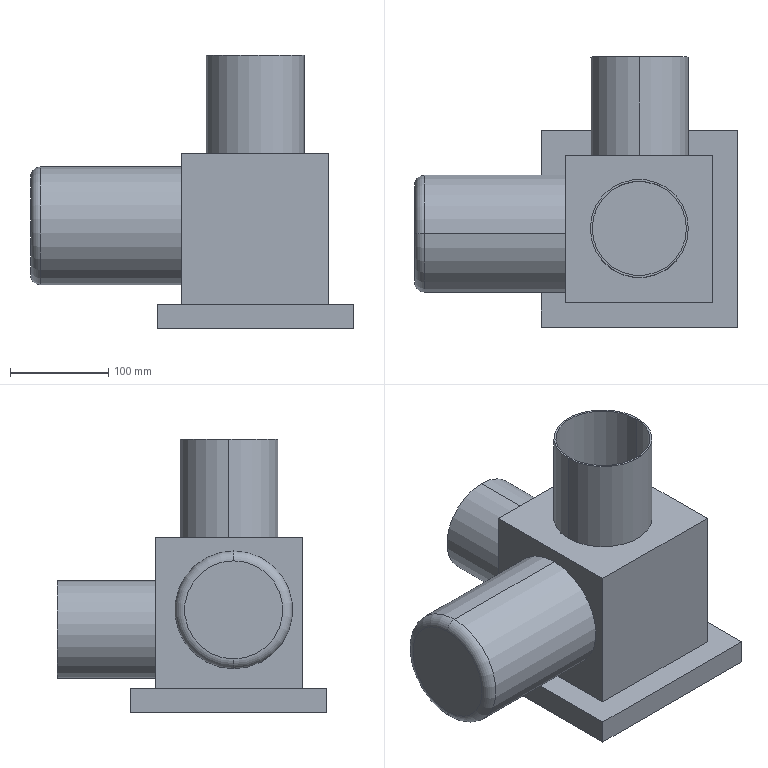Part | SolidWorks | features ICE 5, Extrusion 1, Fillet 1 | 1 solid | 28 faces | box 329 x 275 x 279 mm | volume 6409711 mm3 | plane 16 | cylinder 10 | torus 2 | commonest cylinder face diameters 100 x4 90 x2 96 x2 120 x2
STEP:
#1=CARTESIAN_POINT('',(-48.,0.,179.));
#2=VERTEX_POINT('',#1);
#3=CARTESIAN_POINT('',(48.,0.,179.));
#4=VERTEX_POINT('',#3);
#5=CARTESIAN_POINT('',(0.,0.,179.));
#6=DIRECTION('',(0.,0.,1.));
#7=DIRECTION('',(-1.,0.,0.));
#8=AXIS2_PLACEMENT_3D('',#5,#6,#7);
#9=CIRCLE('',#8,48.);
#10=EDGE_CURVE('',#2,#4,#9,.T.);
#11=ORIENTED_EDGE('',*,*,#10,.F.);
#12=CARTESIAN_POINT('',(-48.,0.,279.));
#13=VERTEX_POINT('',#12);
#14=CARTESIAN_POINT('',(-48.,0.,43.235));
#15=DIRECTION('',(0.,0.,1.));
#16=VECTOR('',#15,1000.);
#17=LINE('',#14,#16);
#18=EDGE_CURVE('',#2,#13,#17,.T.);
#19=ORIENTED_EDGE('',*,*,#18,.T.);
#20=CARTESIAN_POINT('',(48.,0.,279.));
#21=VERTEX_POINT('',#20);
#22=CARTESIAN_POINT('',(0.,0.,279.));
#23=DIRECTION('',(0.,0.,1.));
#24=DIRECTION('',(1.,0.,0.));
#25=AXIS2_PLACEMENT_3D('',#22,#23,#24);
#26=CIRCLE('',#25,48.);
#27=EDGE_CURVE('',#13,#21,#26,.T.);
#28=ORIENTED_EDGE('',*,*,#27,.T.);
#29=CARTESIAN_POINT('',(48.,0.,43.235));
#30=DIRECTION('',(0.,0.,1.));
#31=VECTOR('',#30,1000.);
#32=LINE('',#29,#31);
#33=EDGE_CURVE('',#4,#21,#32,.T.);
#34=ORIENTED_EDGE('',*,*,#33,.F.);
#35=EDGE_LOOP('',(#11,#19,#28,#34));
#36=FACE_OUTER_BOUND('',#35,.T.);
#37=CARTESIAN_POINT('',(0.,0.,43.235));
#38=DIRECTION('',(0.,0.,1.));
#39=DIRECTION('',(1.,0.,0.));
#40=AXIS2_PLACEMENT_3D('',#37,#38,#39);
#41=CYLINDRICAL_SURFACE('',#40,48.);
#42=ADVANCED_FACE('',(#36),#41,.F.);
#43=CARTESIAN_POINT('',(0.,175.,40.));
#44=VERTEX_POINT('',#43);
#45=CARTESIAN_POINT('',(0.,175.,130.));
#46=VERTEX_POINT('',#45);
#47=CARTESIAN_POINT('',(0.,175.,85.));
#48=DIRECTION('',(0.,1.,0.));
#49=DIRECTION('',(0.,0.,1.));
#50=AXIS2_PLACEMENT_3D('',#47,#48,#49);
#51=CIRCLE('',#50,45.);
#52=EDGE_CURVE('',#44,#46,#51,.T.);
#53=ORIENTED_EDGE('',*,*,#52,.T.);
#54=CARTESIAN_POINT('',(0.,75.,130.));
#55=VERTEX_POINT('',#54);
#56=CARTESIAN_POINT('',(0.,175.,130.));
#57=DIRECTION('',(0.,-1.,0.));
#58=VECTOR('',#57,1000.);
#59=LINE('',#56,#58);
#60=EDGE_CURVE('',#46,#55,#59,.T.);
#61=ORIENTED_EDGE('',*,*,#60,.T.);
#62=CARTESIAN_POINT('',(0.,75.,40.));
#63=VERTEX_POINT('',#62);
#64=CARTESIAN_POINT('',(0.,75.,85.));
#65=DIRECTION('',(0.,1.,0.));
#66=DIRECTION('',(0.,0.,1.));
#67=AXIS2_PLACEMENT_3D('',#64,#65,#66);
#68=CIRCLE('',#67,45.);
#69=EDGE_CURVE('',#63,#55,#68,.T.);
#70=ORIENTED_EDGE('',*,*,#69,.F.);
#71=CARTESIAN_POINT('',(0.,175.,40.));
#72=DIRECTION('',(0.,-1.,0.));
#73=VECTOR('',#72,1000.);
#74=LINE('',#71,#73);
#75=EDGE_CURVE('',#44,#63,#74,.T.);
#76=ORIENTED_EDGE('',*,*,#75,.F.);
#77=EDGE_LOOP('',(#53,#61,#70,#76));
#78=FACE_OUTER_BOUND('',#77,.T.);
#79=CARTESIAN_POINT('',(0.,175.,85.));
#80=DIRECTION('',(0.,-1.,0.));
#81=DIRECTION('',(0.,0.,-1.));
#82=AXIS2_PLACEMENT_3D('',#79,#80,#81);
#83=CYLINDRICAL_SURFACE('',#82,45.);
#84=ADVANCED_FACE('',(#78),#83,.F.);
#85=CARTESIAN_POINT('',(0.,175.,135.));
#86=VERTEX_POINT('',#85);
#87=CARTESIAN_POINT('',(0.,175.,35.));
#88=VERTEX_POINT('',#87);
#89=CARTESIAN_POINT('',(0.,175.,85.));
#90=DIRECTION('',(0.,1.,0.));
#91=DIRECTION('',(0.,0.,1.));
#92=AXIS2_PLACEMENT_3D('',#89,#90,#91);
#93=CIRCLE('',#92,50.);
#94=EDGE_CURVE('',#86,#88,#93,.T.);
#95=ORIENTED_EDGE('',*,*,#94,.F.);
#96=CARTESIAN_POINT('',(0.,75.,135.));
#97=VERTEX_POINT('',#96);
#98=CARTESIAN_POINT('',(0.,175.,135.));
#99=DIRECTION('',(0.,-1.,0.));
#100=VECTOR('',#99,1000.);
#101=LINE('',#98,#100);
#102=EDGE_CURVE('',#86,#97,#101,.T.);
#103=ORIENTED_EDGE('',*,*,#102,.T.);
#104=CARTESIAN_POINT('',(0.,75.,35.));
#105=VERTEX_POINT('',#104);
#106=CARTESIAN_POINT('',(0.,75.,85.));
#107=DIRECTION('',(0.,1.,0.));
#108=DIRECTION('',(0.,0.,-1.));
#109=AXIS2_PLACEMENT_3D('',#106,#107,#108);
#110=CIRCLE('',#109,50.);
#111=EDGE_CURVE('',#97,#105,#110,.T.);
#112=ORIENTED_EDGE('',*,*,#111,.T.);
#113=CARTESIAN_POINT('',(0.,175.,35.));
#114=DIRECTION('',(0.,-1.,0.));
#115=VECTOR('',#114,1000.);
#116=LINE('',#113,#115);
#117=EDGE_CURVE('',#88,#105,#116,.T.);
#118=ORIENTED_EDGE('',*,*,#117,.F.);
#119=EDGE_LOOP('',(#95,#103,#112,#118));
#120=FACE_OUTER_BOUND('',#119,.T.);
#121=CARTESIAN_POINT('',(0.,175.,85.));
#122=DIRECTION('',(0.,-1.,0.));
#123=DIRECTION('',(0.,0.,-1.));
#124=AXIS2_PLACEMENT_3D('',#121,#122,#123);
#125=CYLINDRICAL_SURFACE('',#124,50.);
#126=ADVANCED_FACE('',(#120),#125,.T.);
#127=CARTESIAN_POINT('',(50.,0.,279.));
#128=VERTEX_POINT('',#127);
#129=CARTESIAN_POINT('',(-50.,0.,279.));
#130=VERTEX_POINT('',#129);
#131=CARTESIAN_POINT('',(0.,0.,279.));
#132=DIRECTION('',(0.,0.,1.));
#133=DIRECTION('',(1.,0.,0.));
#134=AXIS2_PLACEMENT_3D('',#131,#132,#133);
#135=CIRCLE('',#134,50.);
#136=EDGE_CURVE('',#128,#130,#135,.T.);
#137=ORIENTED_EDGE('',*,*,#136,.F.);
#138=CARTESIAN_POINT('',(50.,0.,179.));
#139=VERTEX_POINT('',#138);
#140=CARTESIAN_POINT('',(50.,0.,279.));
#141=DIRECTION('',(0.,0.,-1.));
#142=VECTOR('',#141,1000.);
#143=LINE('',#140,#142);
#144=EDGE_CURVE('',#128,#139,#143,.T.);
#145=ORIENTED_EDGE('',*,*,#144,.T.);
#146=CARTESIAN_POINT('',(-50.,0.,179.));
#147=VERTEX_POINT('',#146);
#148=CARTESIAN_POINT('',(0.,0.,179.));
#149=DIRECTION('',(0.,0.,1.));
#150=DIRECTION('',(1.,0.,0.));
#151=AXIS2_PLACEMENT_3D('',#148,#149,#150);
#152=CIRCLE('',#151,50.);
#153=EDGE_CURVE('',#139,#147,#152,.T.);
#154=ORIENTED_EDGE('',*,*,#153,.T.);
#155=CARTESIAN_POINT('',(-50.,0.,279.));
#156=DIRECTION('',(0.,0.,-1.));
#157=VECTOR('',#156,1000.);
#158=LINE('',#155,#157);
#159=EDGE_CURVE('',#130,#147,#158,.T.);
#160=ORIENTED_EDGE('',*,*,#159,.F.);
#161=EDGE_LOOP('',(#137,#145,#154,#160));
#162=FACE_OUTER_BOUND('',#161,.T.);
#163=CARTESIAN_POINT('',(0.,0.,279.));
#164=DIRECTION('',(0.,0.,-1.));
#165=DIRECTION('',(-1.,0.,0.));
#166=AXIS2_PLACEMENT_3D('',#163,#164,#165);
#167=CYLINDRICAL_SURFACE('',#166,50.);
#168=ADVANCED_FACE('',(#162),#167,.T.);
#169=CARTESIAN_POINT('',(-229.,-5.,155.));
#170=VERTEX_POINT('',#169);
#171=CARTESIAN_POINT('',(-229.,-5.,55.));
#172=VERTEX_POINT('',#171);
#173=CARTESIAN_POINT('',(-229.,-5.,105.));
#174=DIRECTION('',(-1.,0.,0.));
#175=DIRECTION('',(0.,0.,-1.));
#176=AXIS2_PLACEMENT_3D('',#173,#174,#175);
#177=CIRCLE('',#176,50.);
#178=EDGE_CURVE('',#170,#172,#177,.T.);
#179=ORIENTED_EDGE('',*,*,#178,.F.);
#180=CARTESIAN_POINT('',(-219.,-5.,165.));
#181=VERTEX_POINT('',#180);
#182=CARTESIAN_POINT('',(-219.,-5.,155.));
#183=DIRECTION('',(0.,1.,0.));
#184=DIRECTION('',(0.,0.,1.));
#185=AXIS2_PLACEMENT_3D('',#182,#183,#184);
#186=CIRCLE('',#185,10.);
#187=EDGE_CURVE('',#170,#181,#186,.T.);
#188=ORIENTED_EDGE('',*,*,#187,.T.);
#189=CARTESIAN_POINT('',(-219.,-5.,45.));
#190=VERTEX_POINT('',#189);
#191=CARTESIAN_POINT('',(-219.,-5.,105.));
#192=DIRECTION('',(1.,0.,0.));
#193=DIRECTION('',(0.,0.,-1.));
#194=AXIS2_PLACEMENT_3D('',#191,#192,#193);
#195=CIRCLE('',#194,60.);
#196=EDGE_CURVE('',#190,#181,#195,.T.);
#197=ORIENTED_EDGE('',*,*,#196,.F.);
#198=CARTESIAN_POINT('',(-219.,-5.,55.));
#199=DIRECTION('',(0.,-1.,0.));
#200=DIRECTION('',(0.,0.,-1.));
#201=AXIS2_PLACEMENT_3D('',#198,#199,#200);
#202=CIRCLE('',#201,10.);
#203=EDGE_CURVE('',#172,#190,#202,.T.);
#204=ORIENTED_EDGE('',*,*,#203,.F.);
#205=EDGE_LOOP('',(#179,#188,#197,#204));
#206=FACE_OUTER_BOUND('',#205,.T.);
#207=CARTESIAN_POINT('',(-219.,-5.,105.));
#208=DIRECTION('',(1.,0.,0.));
#209=DIRECTION('',(0.,0.,-1.));
#210=AXIS2_PLACEMENT_3D('',#207,#208,#209);
#211=TOROIDAL_SURFACE('',#210,50.,10.);
#212=ADVANCED_FACE('',(#206),#211,.T.);
#213=ORIENTED_EDGE('',*,*,#196,.T.);
#214=CARTESIAN_POINT('',(-75.,-5.,165.));
#215=VERTEX_POINT('',#214);
#216=CARTESIAN_POINT('',(-229.,-5.,165.));
#217=DIRECTION('',(1.,0.,0.));
#218=VECTOR('',#217,1000.);
#219=LINE('',#216,#218);
#220=EDGE_CURVE('',#181,#215,#219,.T.);
#221=ORIENTED_EDGE('',*,*,#220,.T.);
#222=CARTESIAN_POINT('',(-75.,-5.,45.));
#223=VERTEX_POINT('',#222);
#224=CARTESIAN_POINT('',(-75.,-5.,105.));
#225=DIRECTION('',(1.,0.,0.));
#226=DIRECTION('',(0.,0.,-1.));
#227=AXIS2_PLACEMENT_3D('',#224,#225,#226);
#228=CIRCLE('',#227,60.);
#229=EDGE_CURVE('',#223,#215,#228,.T.);
#230=ORIENTED_EDGE('',*,*,#229,.F.);
#231=CARTESIAN_POINT('',(-229.,-5.,45.));
#232=DIRECTION('',(1.,0.,0.));
#233=VECTOR('',#232,1000.);
#234=LINE('',#231,#233);
#235=EDGE_CURVE('',#190,#223,#234,.T.);
#236=ORIENTED_EDGE('',*,*,#235,.F.);
#237=EDGE_LOOP('',(#213,#221,#230,#236));
#238=FACE_OUTER_BOUND('',#237,.T.);
#239=CARTESIAN_POINT('',(-229.,-5.,105.));
#240=DIRECTION('',(1.,0.,0.));
#241=DIRECTION('',(0.,0.,-1.));
#242=AXIS2_PLACEMENT_3D('',#239,#240,#241);
#243=CYLINDRICAL_SURFACE('',#242,60.);
#244=ADVANCED_FACE('',(#238),#243,.T.);
#245=CARTESIAN_POINT('',(100.,-100.,25.));
#246=VERTEX_POINT('',#245);
#247=CARTESIAN_POINT('',(100.,100.,25.));
#248=VERTEX_POINT('',#247);
#249=CARTESIAN_POINT('',(100.,-100.,25.));
#250=DIRECTION('',(0.,1.,0.));
#251=VECTOR('',#250,1000.);
#252=LINE('',#249,#251);
#253=EDGE_CURVE('',#246,#248,#252,.T.);
#254=ORIENTED_EDGE('',*,*,#253,.T.);
#255=CARTESIAN_POINT('',(-100.,100.,25.));
#256=VERTEX_POINT('',#255);
#257=CARTESIAN_POINT('',(-100.,100.,25.));
#258=DIRECTION('',(-1.,0.,0.));
#259=VECTOR('',#258,1000.);
#260=LINE('',#257,#259);
#261=EDGE_CURVE('',#248,#256,#260,.T.);
#262=ORIENTED_EDGE('',*,*,#261,.T.);
#263=CARTESIAN_POINT('',(-100.,-100.,25.));
#264=VERTEX_POINT('',#263);
#265=CARTESIAN_POINT('',(-100.,-100.,25.));
#266=DIRECTION('',(0.,-1.,0.));
#267=VECTOR('',#266,1000.);
#268=LINE('',#265,#267);
#269=EDGE_CURVE('',#256,#264,#268,.T.);
#270=ORIENTED_EDGE('',*,*,#269,.T.);
#271=CARTESIAN_POINT('',(-100.,-100.,25.));
#272=DIRECTION('',(1.,0.,0.));
#273=VECTOR('',#272,1000.);
#274=LINE('',#271,#273);
#275=EDGE_CURVE('',#264,#246,#274,.T.);
#276=ORIENTED_EDGE('',*,*,#275,.T.);
#277=EDGE_LOOP('',(#254,#262,#270,#276));
#278=FACE_OUTER_BOUND('',#277,.T.);
#279=CARTESIAN_POINT('',(75.,-75.,25.));
#280=VERTEX_POINT('',#279);
#281=CARTESIAN_POINT('',(75.,75.,25.));
#282=VERTEX_POINT('',#281);
#283=CARTESIAN_POINT('',(75.,-75.,25.));
#284=DIRECTION('',(0.,1.,0.));
#285=VECTOR('',#284,1000.);
#286=LINE('',#283,#285);
#287=EDGE_CURVE('',#280,#282,#286,.T.);
#288=ORIENTED_EDGE('',*,*,#287,.F.);
#289=CARTESIAN_POINT('',(-75.,-75.,25.));
#290=VERTEX_POINT('',#289);
#291=CARTESIAN_POINT('',(-75.,-75.,25.));
#292=DIRECTION('',(1.,0.,0.));
#293=VECTOR('',#292,1000.);
#294=LINE('',#291,#293);
#295=EDGE_CURVE('',#290,#280,#294,.T.);
#296=ORIENTED_EDGE('',*,*,#295,.F.);
#297=CARTESIAN_POINT('',(-75.,75.,25.));
#298=VERTEX_POINT('',#297);
#299=CARTESIAN_POINT('',(-75.,-75.,25.));
#300=DIRECTION('',(0.,-1.,0.));
#301=VECTOR('',#300,1000.);
#302=LINE('',#299,#301);
#303=EDGE_CURVE('',#298,#290,#302,.T.);
#304=ORIENTED_EDGE('',*,*,#303,.F.);
#305=CARTESIAN_POINT('',(-75.,75.,25.));
#306=DIRECTION('',(-1.,0.,0.));
#307=VECTOR('',#306,1000.);
#308=LINE('',#305,#307);
#309=EDGE_CURVE('',#282,#298,#308,.T.);
#310=ORIENTED_EDGE('',*,*,#309,.F.);
#311=EDGE_LOOP('',(#288,#296,#304,#310));
#312=FACE_BOUND('',#311,.T.);
#313=CARTESIAN_POINT('',(0.,0.,25.));
#314=DIRECTION('',(0.,0.,-1.));
#315=DIRECTION('',(-1.,0.,0.));
#316=AXIS2_PLACEMENT_3D('',#313,#314,#315);
#317=PLANE('',#316);
#318=ADVANCED_FACE('',(#278,#312),#317,.F.);
#319=CARTESIAN_POINT('',(100.,-100.,0.));
#320=VERTEX_POINT('',#319);
#321=CARTESIAN_POINT('',(100.,100.,0.));
#322=VERTEX_POINT('',#321);
#323=CARTESIAN_POINT('',(100.,-100.,0.));
#324=DIRECTION('',(0.,1.,0.));
#325=VECTOR('',#324,1000.);
#326=LINE('',#323,#325);
#327=EDGE_CURVE('',#320,#322,#326,.T.);
#328=ORIENTED_EDGE('',*,*,#327,.T.);
#329=CARTESIAN_POINT('',(100.,100.,25.));
#330=DIRECTION('',(0.,0.,-1.));
#331=VECTOR('',#330,1000.);
#332=LINE('',#329,#331);
#333=EDGE_CURVE('',#248,#322,#332,.T.);
#334=ORIENTED_EDGE('',*,*,#333,.F.);
#335=ORIENTED_EDGE('',*,*,#253,.F.);
#336=CARTESIAN_POINT('',(100.,-100.,25.));
#337=DIRECTION('',(0.,0.,-1.));
#338=VECTOR('',#337,1000.);
#339=LINE('',#336,#338);
#340=EDGE_CURVE('',#246,#320,#339,.T.);
#341=ORIENTED_EDGE('',*,*,#340,.T.);
#342=EDGE_LOOP('',(#328,#334,#335,#341));
#343=FACE_OUTER_BOUND('',#342,.T.);
#344=CARTESIAN_POINT('',(100.,-100.,25.));
#345=DIRECTION('',(-1.,0.,0.));
#346=DIRECTION('',(0.,0.,1.));
#347=AXIS2_PLACEMENT_3D('',#344,#345,#346);
#348=PLANE('',#347);
#349=ADVANCED_FACE('',(#343),#348,.F.);
#350=CARTESIAN_POINT('',(-100.,100.,0.));
#351=VERTEX_POINT('',#350);
#352=CARTESIAN_POINT('',(-100.,100.,0.));
#353=DIRECTION('',(-1.,0.,0.));
#354=VECTOR('',#353,1000.);
#355=LINE('',#352,#354);
#356=EDGE_CURVE('',#322,#351,#355,.T.);
#357=ORIENTED_EDGE('',*,*,#356,.T.);
#358=CARTESIAN_POINT('',(-100.,100.,25.));
#359=DIRECTION('',(0.,0.,-1.));
#360=VECTOR('',#359,1000.);
#361=LINE('',#358,#360);
#362=EDGE_CURVE('',#256,#351,#361,.T.);
#363=ORIENTED_EDGE('',*,*,#362,.F.);
#364=ORIENTED_EDGE('',*,*,#261,.F.);
#365=ORIENTED_EDGE('',*,*,#333,.T.);
#366=EDGE_LOOP('',(#357,#363,#364,#365));
#367=FACE_OUTER_BOUND('',#366,.T.);
#368=CARTESIAN_POINT('',(-100.,100.,25.));
#369=DIRECTION('',(0.,-1.,0.));
#370=DIRECTION('',(0.,0.,-1.));
#371=AXIS2_PLACEMENT_3D('',#368,#369,#370);
#372=PLANE('',#371);
#373=ADVANCED_FACE('',(#367),#372,.F.);
#374=CARTESIAN_POINT('',(-100.,-100.,0.));
#375=VERTEX_POINT('',#374);
#376=CARTESIAN_POINT('',(-100.,-100.,0.));
#377=DIRECTION('',(0.,-1.,0.));
#378=VECTOR('',#377,1000.);
#379=LINE('',#376,#378);
#380=EDGE_CURVE('',#351,#375,#379,.T.);
#381=ORIENTED_EDGE('',*,*,#380,.T.);
#382=CARTESIAN_POINT('',(-100.,-100.,25.));
#383=DIRECTION('',(0.,0.,-1.));
#384=VECTOR('',#383,1000.);
#385=LINE('',#382,#384);
#386=EDGE_CURVE('',#264,#375,#385,.T.);
#387=ORIENTED_EDGE('',*,*,#386,.F.);
#388=ORIENTED_EDGE('',*,*,#269,.F.);
#389=ORIENTED_EDGE('',*,*,#362,.T.);
#390=EDGE_LOOP('',(#381,#387,#388,#389));
#391=FACE_OUTER_BOUND('',#390,.T.);
#392=CARTESIAN_POINT('',(-100.,-100.,25.));
#393=DIRECTION('',(1.,0.,0.));
#394=DIRECTION('',(0.,0.,-1.));
#395=AXIS2_PLACEMENT_3D('',#392,#393,#394);
#396=PLANE('',#395);
#397=ADVANCED_FACE('',(#391),#396,.F.);
#398=CARTESIAN_POINT('',(-100.,-100.,0.));
#399=DIRECTION('',(1.,0.,0.));
#400=VECTOR('',#399,1000.);
#401=LINE('',#398,#400);
#402=EDGE_CURVE('',#375,#320,#401,.T.);
#403=ORIENTED_EDGE('',*,*,#402,.T.);
#404=ORIENTED_EDGE('',*,*,#340,.F.);
#405=ORIENTED_EDGE('',*,*,#275,.F.);
#406=ORIENTED_EDGE('',*,*,#386,.T.);
#407=EDGE_LOOP('',(#403,#404,#405,#406));
#408=FACE_OUTER_BOUND('',#407,.T.);
#409=CARTESIAN_POINT('',(-100.,-100.,25.));
#410=DIRECTION('',(0.,1.,0.));
#411=DIRECTION('',(0.,0.,1.));
#412=AXIS2_PLACEMENT_3D('',#409,#410,#411);
#413=PLANE('',#412);
#414=ADVANCED_FACE('',(#408),#413,.F.);
#415=ORIENTED_EDGE('',*,*,#327,.F.);
#416=ORIENTED_EDGE('',*,*,#402,.F.);
#417=ORIENTED_EDGE('',*,*,#380,.F.);
#418=ORIENTED_EDGE('',*,*,#356,.F.);
#419=EDGE_LOOP('',(#415,#416,#417,#418));
#420=FACE_OUTER_BOUND('',#419,.T.);
#421=CARTESIAN_POINT('',(0.,0.,0.));
#422=DIRECTION('',(0.,0.,-1.));
#423=DIRECTION('',(-1.,0.,0.));
#424=AXIS2_PLACEMENT_3D('',#421,#422,#423);
#425=PLANE('',#424);
#426=ADVANCED_FACE('',(#420),#425,.T.);
#427=ORIENTED_EDGE('',*,*,#287,.T.);
#428=CARTESIAN_POINT('',(75.,75.,179.));
#429=VERTEX_POINT('',#428);
#430=CARTESIAN_POINT('',(75.,75.,179.));
#431=DIRECTION('',(0.,0.,-1.));
#432=VECTOR('',#431,1000.);
#433=LINE('',#430,#432);
#434=EDGE_CURVE('',#429,#282,#433,.T.);
#435=ORIENTED_EDGE('',*,*,#434,.F.);
#436=CARTESIAN_POINT('',(75.,-75.,179.));
#437=VERTEX_POINT('',#436);
#438=CARTESIAN_POINT('',(75.,-75.,179.));
#439=DIRECTION('',(0.,1.,0.));
#440=VECTOR('',#439,1000.);
#441=LINE('',#438,#440);
#442=EDGE_CURVE('',#437,#429,#441,.T.);
#443=ORIENTED_EDGE('',*,*,#442,.F.);
#444=CARTESIAN_POINT('',(75.,-75.,179.));
#445=DIRECTION('',(0.,0.,-1.));
#446=VECTOR('',#445,1000.);
#447=LINE('',#444,#446);
#448=EDGE_CURVE('',#437,#280,#447,.T.);
#449=ORIENTED_EDGE('',*,*,#448,.T.);
#450=EDGE_LOOP('',(#427,#435,#443,#449));
#451=FACE_OUTER_BOUND('',#450,.T.);
#452=CARTESIAN_POINT('',(75.,-75.,179.));
#453=DIRECTION('',(-1.,0.,0.));
#454=DIRECTION('',(0.,0.,1.));
#455=AXIS2_PLACEMENT_3D('',#452,#453,#454);
#456=PLANE('',#455);
#457=ADVANCED_FACE('',(#451),#456,.F.);
#458=CARTESIAN_POINT('',(0.,75.,85.));
#459=DIRECTION('',(0.,1.,0.));
#460=DIRECTION('',(0.,0.,-1.));
#461=AXIS2_PLACEMENT_3D('',#458,#459,#460);
#462=CIRCLE('',#461,50.);
#463=EDGE_CURVE('',#105,#97,#462,.T.);
#464=ORIENTED_EDGE('',*,*,#463,.F.);
#465=ORIENTED_EDGE('',*,*,#111,.F.);
#466=EDGE_LOOP('',(#464,#465));
#467=FACE_BOUND('',#466,.T.);
#468=ORIENTED_EDGE('',*,*,#309,.T.);
#469=CARTESIAN_POINT('',(-75.,75.,179.));
#470=VERTEX_POINT('',#469);
#471=CARTESIAN_POINT('',(-75.,75.,179.));
#472=DIRECTION('',(0.,0.,-1.));
#473=VECTOR('',#472,1000.);
#474=LINE('',#471,#473);
#475=EDGE_CURVE('',#470,#298,#474,.T.);
#476=ORIENTED_EDGE('',*,*,#475,.F.);
#477=CARTESIAN_POINT('',(-75.,75.,179.));
#478=DIRECTION('',(-1.,0.,0.));
#479=VECTOR('',#478,1000.);
#480=LINE('',#477,#479);
#481=EDGE_CURVE('',#429,#470,#480,.T.);
#482=ORIENTED_EDGE('',*,*,#481,.F.);
#483=ORIENTED_EDGE('',*,*,#434,.T.);
#484=EDGE_LOOP('',(#468,#476,#482,#483));
#485=FACE_OUTER_BOUND('',#484,.T.);
#486=CARTESIAN_POINT('',(-75.,75.,179.));
#487=DIRECTION('',(0.,-1.,0.));
#488=DIRECTION('',(0.,0.,-1.));
#489=AXIS2_PLACEMENT_3D('',#486,#487,#488);
#490=PLANE('',#489);
#491=ADVANCED_FACE('',(#467,#485),#490,.F.);
#492=ORIENTED_EDGE('',*,*,#229,.T.);
#493=CARTESIAN_POINT('',(-75.,-5.,105.));
#494=DIRECTION('',(1.,0.,0.));
#495=DIRECTION('',(0.,0.,-1.));
#496=AXIS2_PLACEMENT_3D('',#493,#494,#495);
#497=CIRCLE('',#496,60.);
#498=EDGE_CURVE('',#215,#223,#497,.T.);
#499=ORIENTED_EDGE('',*,*,#498,.T.);
#500=EDGE_LOOP('',(#492,#499));
#501=FACE_BOUND('',#500,.T.);
#502=ORIENTED_EDGE('',*,*,#303,.T.);
#503=CARTESIAN_POINT('',(-75.,-75.,179.));
#504=VERTEX_POINT('',#503);
#505=CARTESIAN_POINT('',(-75.,-75.,179.));
#506=DIRECTION('',(0.,0.,-1.));
#507=VECTOR('',#506,1000.);
#508=LINE('',#505,#507);
#509=EDGE_CURVE('',#504,#290,#508,.T.);
#510=ORIENTED_EDGE('',*,*,#509,.F.);
#511=CARTESIAN_POINT('',(-75.,-75.,179.));
#512=DIRECTION('',(0.,-1.,0.));
#513=VECTOR('',#512,1000.);
#514=LINE('',#511,#513);
#515=EDGE_CURVE('',#470,#504,#514,.T.);
#516=ORIENTED_EDGE('',*,*,#515,.F.);
#517=ORIENTED_EDGE('',*,*,#475,.T.);
#518=EDGE_LOOP('',(#502,#510,#516,#517));
#519=FACE_OUTER_BOUND('',#518,.T.);
#520=CARTESIAN_POINT('',(-75.,-75.,179.));
#521=DIRECTION('',(1.,0.,0.));
#522=DIRECTION('',(0.,0.,-1.));
#523=AXIS2_PLACEMENT_3D('',#520,#521,#522);
#524=PLANE('',#523);
#525=ADVANCED_FACE('',(#501,#519),#524,.F.);
#526=ORIENTED_EDGE('',*,*,#295,.T.);
#527=ORIENTED_EDGE('',*,*,#448,.F.);
#528=CARTESIAN_POINT('',(-75.,-75.,179.));
#529=DIRECTION('',(1.,0.,0.));
#530=VECTOR('',#529,1000.);
#531=LINE('',#528,#530);
#532=EDGE_CURVE('',#504,#437,#531,.T.);
#533=ORIENTED_EDGE('',*,*,#532,.F.);
#534=ORIENTED_EDGE('',*,*,#509,.T.);
#535=EDGE_LOOP('',(#526,#527,#533,#534));
#536=FACE_OUTER_BOUND('',#535,.T.);
#537=CARTESIAN_POINT('',(-75.,-75.,179.));
#538=DIRECTION('',(0.,1.,0.));
#539=DIRECTION('',(0.,0.,1.));
#540=AXIS2_PLACEMENT_3D('',#537,#538,#539);
#541=PLANE('',#540);
#542=ADVANCED_FACE('',(#536),#541,.F.);
#543=CARTESIAN_POINT('',(0.,0.,179.));
#544=DIRECTION('',(0.,0.,1.));
#545=DIRECTION('',(1.,0.,0.));
#546=AXIS2_PLACEMENT_3D('',#543,#544,#545);
#547=CIRCLE('',#546,50.);
#548=EDGE_CURVE('',#147,#139,#547,.T.);
#549=ORIENTED_EDGE('',*,*,#548,.F.);
#550=ORIENTED_EDGE('',*,*,#153,.F.);
#551=EDGE_LOOP('',(#549,#550));
#552=FACE_BOUND('',#551,.T.);
#553=ORIENTED_EDGE('',*,*,#442,.T.);
#554=ORIENTED_EDGE('',*,*,#481,.T.);
#555=ORIENTED_EDGE('',*,*,#515,.T.);
#556=ORIENTED_EDGE('',*,*,#532,.T.);
#557=EDGE_LOOP('',(#553,#554,#555,#556));
#558=FACE_OUTER_BOUND('',#557,.T.);
#559=CARTESIAN_POINT('',(0.,0.,179.));
#560=DIRECTION('',(0.,0.,-1.));
#561=DIRECTION('',(-1.,0.,0.));
#562=AXIS2_PLACEMENT_3D('',#559,#560,#561);
#563=PLANE('',#562);
#564=ADVANCED_FACE('',(#552,#558),#563,.F.);
#565=ORIENTED_EDGE('',*,*,#220,.F.);
#566=CARTESIAN_POINT('',(-219.,-5.,105.));
#567=DIRECTION('',(1.,0.,0.));
#568=DIRECTION('',(0.,0.,-1.));
#569=AXIS2_PLACEMENT_3D('',#566,#567,#568);
#570=CIRCLE('',#569,60.);
#571=EDGE_CURVE('',#181,#190,#570,.T.);
#572=ORIENTED_EDGE('',*,*,#571,.T.);
#573=ORIENTED_EDGE('',*,*,#235,.T.);
#574=ORIENTED_EDGE('',*,*,#498,.F.);
#575=EDGE_LOOP('',(#565,#572,#573,#574));
#576=FACE_OUTER_BOUND('',#575,.T.);
#577=CARTESIAN_POINT('',(-229.,-5.,105.));
#578=DIRECTION('',(1.,0.,0.));
#579=DIRECTION('',(0.,0.,-1.));
#580=AXIS2_PLACEMENT_3D('',#577,#578,#579);
#581=CYLINDRICAL_SURFACE('',#580,60.);
#582=ADVANCED_FACE('',(#576),#581,.T.);
#583=CARTESIAN_POINT('',(-229.,-5.,105.));
#584=DIRECTION('',(-1.,0.,0.));
#585=DIRECTION('',(0.,0.,-1.));
#586=AXIS2_PLACEMENT_3D('',#583,#584,#585);
#587=CIRCLE('',#586,50.);
#588=EDGE_CURVE('',#172,#170,#587,.T.);
#589=ORIENTED_EDGE('',*,*,#588,.T.);
#590=ORIENTED_EDGE('',*,*,#178,.T.);
#591=EDGE_LOOP('',(#589,#590));
#592=FACE_OUTER_BOUND('',#591,.T.);
#593=CARTESIAN_POINT('',(-229.,-5.,105.));
#594=DIRECTION('',(1.,0.,0.));
#595=DIRECTION('',(0.,0.,-1.));
#596=AXIS2_PLACEMENT_3D('',#593,#594,#595);
#597=PLANE('',#596);
#598=ADVANCED_FACE('',(#592),#597,.F.);
#599=ORIENTED_EDGE('',*,*,#187,.F.);
#600=ORIENTED_EDGE('',*,*,#588,.F.);
#601=ORIENTED_EDGE('',*,*,#203,.T.);
#602=ORIENTED_EDGE('',*,*,#571,.F.);
#603=EDGE_LOOP('',(#599,#600,#601,#602));
#604=FACE_OUTER_BOUND('',#603,.T.);
#605=CARTESIAN_POINT('',(-219.,-5.,105.));
#606=DIRECTION('',(1.,0.,0.));
#607=DIRECTION('',(0.,0.,-1.));
#608=AXIS2_PLACEMENT_3D('',#605,#606,#607);
#609=TOROIDAL_SURFACE('',#608,50.,10.);
#610=ADVANCED_FACE('',(#604),#609,.T.);
#611=ORIENTED_EDGE('',*,*,#144,.F.);
#612=CARTESIAN_POINT('',(0.,0.,279.));
#613=DIRECTION('',(0.,0.,1.));
#614=DIRECTION('',(1.,0.,0.));
#615=AXIS2_PLACEMENT_3D('',#612,#613,#614);
#616=CIRCLE('',#615,50.);
#617=EDGE_CURVE('',#130,#128,#616,.T.);
#618=ORIENTED_EDGE('',*,*,#617,.F.);
#619=ORIENTED_EDGE('',*,*,#159,.T.);
#620=ORIENTED_EDGE('',*,*,#548,.T.);
#621=EDGE_LOOP('',(#611,#618,#619,#620));
#622=FACE_OUTER_BOUND('',#621,.T.);
#623=CARTESIAN_POINT('',(0.,0.,279.));
#624=DIRECTION('',(0.,0.,-1.));
#625=DIRECTION('',(-1.,0.,0.));
#626=AXIS2_PLACEMENT_3D('',#623,#624,#625);
#627=CYLINDRICAL_SURFACE('',#626,50.);
#628=ADVANCED_FACE('',(#622),#627,.T.);
#629=CARTESIAN_POINT('',(0.,0.,279.));
#630=DIRECTION('',(0.,0.,1.));
#631=DIRECTION('',(1.,0.,0.));
#632=AXIS2_PLACEMENT_3D('',#629,#630,#631);
#633=CIRCLE('',#632,48.);
#634=EDGE_CURVE('',#21,#13,#633,.T.);
#635=ORIENTED_EDGE('',*,*,#634,.F.);
#636=ORIENTED_EDGE('',*,*,#27,.F.);
#637=EDGE_LOOP('',(#635,#636));
#638=FACE_BOUND('',#637,.T.);
#639=ORIENTED_EDGE('',*,*,#617,.T.);
#640=ORIENTED_EDGE('',*,*,#136,.T.);
#641=EDGE_LOOP('',(#639,#640));
#642=FACE_OUTER_BOUND('',#641,.T.);
#643=CARTESIAN_POINT('',(0.,0.,279.));
#644=DIRECTION('',(0.,0.,1.));
#645=DIRECTION('',(1.,0.,0.));
#646=AXIS2_PLACEMENT_3D('',#643,#644,#645);
#647=PLANE('',#646);
#648=ADVANCED_FACE('',(#638,#642),#647,.T.);
#649=CARTESIAN_POINT('',(0.,175.,85.));
#650=DIRECTION('',(0.,1.,0.));
#651=DIRECTION('',(0.,0.,1.));
#652=AXIS2_PLACEMENT_3D('',#649,#650,#651);
#653=CIRCLE('',#652,50.);
#654=EDGE_CURVE('',#88,#86,#653,.T.);
#655=ORIENTED_EDGE('',*,*,#654,.T.);
#656=ORIENTED_EDGE('',*,*,#94,.T.);
#657=EDGE_LOOP('',(#655,#656));
#658=FACE_OUTER_BOUND('',#657,.T.);
#659=ORIENTED_EDGE('',*,*,#52,.F.);
#660=CARTESIAN_POINT('',(0.,175.,85.));
#661=DIRECTION('',(0.,1.,0.));
#662=DIRECTION('',(0.,0.,1.));
#663=AXIS2_PLACEMENT_3D('',#660,#661,#662);
#664=CIRCLE('',#663,45.);
#665=EDGE_CURVE('',#46,#44,#664,.T.);
#666=ORIENTED_EDGE('',*,*,#665,.F.);
#667=EDGE_LOOP('',(#659,#666));
#668=FACE_BOUND('',#667,.T.);
#669=CARTESIAN_POINT('',(0.,175.,85.));
#670=DIRECTION('',(0.,1.,0.));
#671=DIRECTION('',(0.,0.,1.));
#672=AXIS2_PLACEMENT_3D('',#669,#670,#671);
#673=PLANE('',#672);
#674=ADVANCED_FACE('',(#658,#668),#673,.T.);
#675=ORIENTED_EDGE('',*,*,#102,.F.);
#676=ORIENTED_EDGE('',*,*,#654,.F.);
#677=ORIENTED_EDGE('',*,*,#117,.T.);
#678=ORIENTED_EDGE('',*,*,#463,.T.);
#679=EDGE_LOOP('',(#675,#676,#677,#678));
#680=FACE_OUTER_BOUND('',#679,.T.);
#681=CARTESIAN_POINT('',(0.,175.,85.));
#682=DIRECTION('',(0.,-1.,0.));
#683=DIRECTION('',(0.,0.,-1.));
#684=AXIS2_PLACEMENT_3D('',#681,#682,#683);
#685=CYLINDRICAL_SURFACE('',#684,50.);
#686=ADVANCED_FACE('',(#680),#685,.T.);
#687=ORIENTED_EDGE('',*,*,#60,.F.);
#688=ORIENTED_EDGE('',*,*,#665,.T.);
#689=ORIENTED_EDGE('',*,*,#75,.T.);
#690=CARTESIAN_POINT('',(0.,75.,85.));
#691=DIRECTION('',(0.,1.,0.));
#692=DIRECTION('',(0.,0.,1.));
#693=AXIS2_PLACEMENT_3D('',#690,#691,#692);
#694=CIRCLE('',#693,45.);
#695=EDGE_CURVE('',#55,#63,#694,.T.);
#696=ORIENTED_EDGE('',*,*,#695,.F.);
#697=EDGE_LOOP('',(#687,#688,#689,#696));
#698=FACE_OUTER_BOUND('',#697,.T.);
#699=CARTESIAN_POINT('',(0.,175.,85.));
#700=DIRECTION('',(0.,-1.,0.));
#701=DIRECTION('',(0.,0.,-1.));
#702=AXIS2_PLACEMENT_3D('',#699,#700,#701);
#703=CYLINDRICAL_SURFACE('',#702,45.);
#704=ADVANCED_FACE('',(#698),#703,.F.);
#705=ORIENTED_EDGE('',*,*,#69,.T.);
#706=ORIENTED_EDGE('',*,*,#695,.T.);
#707=EDGE_LOOP('',(#705,#706));
#708=FACE_OUTER_BOUND('',#707,.T.);
#709=CARTESIAN_POINT('',(-75.,75.,179.));
#710=DIRECTION('',(0.,-1.,0.));
#711=DIRECTION('',(0.,0.,-1.));
#712=AXIS2_PLACEMENT_3D('',#709,#710,#711);
#713=PLANE('',#712);
#714=ADVANCED_FACE('',(#708),#713,.F.);
#715=CARTESIAN_POINT('',(0.,0.,179.));
#716=DIRECTION('',(0.,0.,1.));
#717=DIRECTION('',(-1.,0.,0.));
#718=AXIS2_PLACEMENT_3D('',#715,#716,#717);
#719=CIRCLE('',#718,48.);
#720=EDGE_CURVE('',#4,#2,#719,.T.);
#721=ORIENTED_EDGE('',*,*,#720,.T.);
#722=ORIENTED_EDGE('',*,*,#10,.T.);
#723=EDGE_LOOP('',(#721,#722));
#724=FACE_OUTER_BOUND('',#723,.T.);
#725=CARTESIAN_POINT('',(0.,0.,179.));
#726=DIRECTION('',(0.,0.,-1.));
#727=DIRECTION('',(-1.,0.,0.));
#728=AXIS2_PLACEMENT_3D('',#725,#726,#727);
#729=PLANE('',#728);
#730=ADVANCED_FACE('',(#724),#729,.F.);
#731=ORIENTED_EDGE('',*,*,#18,.F.);
#732=ORIENTED_EDGE('',*,*,#720,.F.);
#733=ORIENTED_EDGE('',*,*,#33,.T.);
#734=ORIENTED_EDGE('',*,*,#634,.T.);
#735=EDGE_LOOP('',(#731,#732,#733,#734));
#736=FACE_OUTER_BOUND('',#735,.T.);
#737=CARTESIAN_POINT('',(0.,0.,43.235));
#738=DIRECTION('',(0.,0.,1.));
#739=DIRECTION('',(1.,0.,0.));
#740=AXIS2_PLACEMENT_3D('',#737,#738,#739);
#741=CYLINDRICAL_SURFACE('',#740,48.);
#742=ADVANCED_FACE('',(#736),#741,.F.);
#743=CLOSED_SHELL('',(#42,#84,#126,#168,#212,#244,#318,#349,#373,#397,#414,#426,#457,#491,#525,#542,#564,#582,#598,#610,#628,#648,#674,#686,#704,#714,#730,#742));
#744=MANIFOLD_SOLID_BREP('',#743);
#745=CARTESIAN_POINT('',(0.,0.,0.));
#746=DIRECTION('',(0.,0.,1.));
#747=DIRECTION('',(1.,0.,0.));
#748=AXIS2_PLACEMENT_3D('',#745,#746,#747);
#749=(LENGTH_UNIT()NAMED_UNIT(*)SI_UNIT(.MILLI.,.METRE.));
#750=UNCERTAINTY_MEASURE_WITH_UNIT(LENGTH_MEASURE(0.00001),#749,'','');
#751=(NAMED_UNIT(*)PLANE_ANGLE_UNIT()SI_UNIT($,.RADIAN.));
#752=(NAMED_UNIT(*)SI_UNIT($,.STERADIAN.)SOLID_ANGLE_UNIT());
#753=(GEOMETRIC_REPRESENTATION_CONTEXT(3)GLOBAL_UNCERTAINTY_ASSIGNED_CONTEXT((#750))GLOBAL_UNIT_ASSIGNED_CONTEXT((#749,#751,#752))REPRESENTATION_CONTEXT('',''));
#754=ADVANCED_BREP_SHAPE_REPRESENTATION('',(#744,#748),#753);